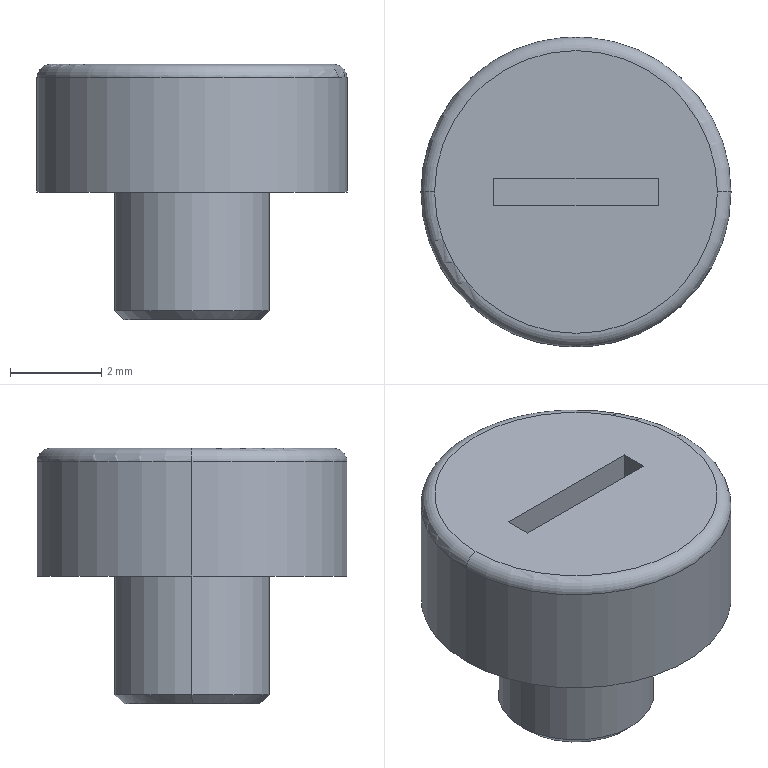Part | STEP file | 4V430C_15_Valve_Button | 1 solid | 16 faces | box 6.8 x 6.8 x 5.6 mm | volume 124.339 mm3 | plane 8 | cylinder 4 | cone 2 | torus 2 | commonest cylinder face diameters 3.4 x2 6.8 x2
STEP:
#1=CARTESIAN_POINT('',(0.,0.,0.));
#2=DIRECTION('',(0.,0.,1.));
#3=DIRECTION('',(1.,0.,0.));
#4=AXIS2_PLACEMENT_3D('',#1,#2,#3);
#5=CARTESIAN_POINT('',(1.5,0.,-2.8));
#6=VERTEX_POINT('',#5);
#7=CARTESIAN_POINT('',(-1.5,0.,-2.8));
#8=VERTEX_POINT('',#7);
#9=CARTESIAN_POINT('',(0.,0.,-2.8));
#10=DIRECTION('',(0.,0.,1.));
#11=DIRECTION('',(1.,0.,0.));
#12=AXIS2_PLACEMENT_3D('',#9,#10,#11);
#13=CIRCLE('',#12,1.5);
#14=CARTESIAN_POINT('',(0.,0.,-2.8));
#15=DIRECTION('',(0.,0.,1.));
#16=DIRECTION('',(1.,0.,0.));
#17=AXIS2_PLACEMENT_3D('',#14,#15,#16);
#18=CONICAL_SURFACE('',#17,1.5,0.7854);
#19=CARTESIAN_POINT('',(0.,0.));
#20=DIRECTION('',(1.,0.));
#21=VECTOR('',#20,1.);
#22=LINE('',#19,#21);
#23=(GEOMETRIC_REPRESENTATION_CONTEXT(2)PARAMETRIC_REPRESENTATION_CONTEXT()REPRESENTATION_CONTEXT('',''));
#24=DEFINITIONAL_REPRESENTATION('',(#22),#23);
#25=PCURVE('',#18,#24);
#26=CARTESIAN_POINT('',(0.,1.5,-2.8));
#27=DIRECTION('',(0.,0.,1.));
#28=DIRECTION('',(1.,0.,0.));
#29=AXIS2_PLACEMENT_3D('',#26,#27,#28);
#30=PLANE('',#29);
#31=CARTESIAN_POINT('',(0.,-1.5));
#32=DIRECTION('',(1.,0.));
#33=AXIS2_PLACEMENT_2D('',#31,#32);
#34=CIRCLE('',#33,1.5);
#35=(GEOMETRIC_REPRESENTATION_CONTEXT(2)PARAMETRIC_REPRESENTATION_CONTEXT()REPRESENTATION_CONTEXT('',''));
#36=DEFINITIONAL_REPRESENTATION('',(#34),#35);
#37=PCURVE('',#30,#36);
#38=SURFACE_CURVE('',#13,(#25,#37),.PCURVE_S1.);
#39=EDGE_CURVE('',#6,#8,#38,.T.);
#40=ORIENTED_EDGE('',*,*,#39,.T.);
#41=CARTESIAN_POINT('',(-1.7,0.,-2.6));
#42=VERTEX_POINT('',#41);
#43=CARTESIAN_POINT('',(-1.5,0.,-2.8));
#44=DIRECTION('',(-0.7071,0.,0.7071));
#45=VECTOR('',#44,1.);
#46=LINE('',#43,#45);
#47=CARTESIAN_POINT('',(3.142,0.));
#48=DIRECTION('',(0.,1.));
#49=VECTOR('',#48,1.);
#50=LINE('',#47,#49);
#51=(GEOMETRIC_REPRESENTATION_CONTEXT(2)PARAMETRIC_REPRESENTATION_CONTEXT()REPRESENTATION_CONTEXT('',''));
#52=DEFINITIONAL_REPRESENTATION('',(#50),#51);
#53=PCURVE('',#18,#52);
#54=CARTESIAN_POINT('',(0.,0.,-2.8));
#55=DIRECTION('',(0.,0.,1.));
#56=DIRECTION('',(1.,0.,0.));
#57=AXIS2_PLACEMENT_3D('',#54,#55,#56);
#58=CONICAL_SURFACE('',#57,1.5,0.7854);
#59=CARTESIAN_POINT('',(3.142,0.));
#60=DIRECTION('',(0.,1.));
#61=VECTOR('',#60,1.);
#62=LINE('',#59,#61);
#63=(GEOMETRIC_REPRESENTATION_CONTEXT(2)PARAMETRIC_REPRESENTATION_CONTEXT()REPRESENTATION_CONTEXT('',''));
#64=DEFINITIONAL_REPRESENTATION('',(#62),#63);
#65=PCURVE('',#58,#64);
#66=SURFACE_CURVE('',#46,(#53,#65),.PCURVE_S1.);
#67=EDGE_CURVE('',#8,#42,#66,.T.);
#68=ORIENTED_EDGE('',*,*,#67,.T.);
#69=CARTESIAN_POINT('',(1.7,0.,-2.6));
#70=VERTEX_POINT('',#69);
#71=CARTESIAN_POINT('',(0.,0.,-2.6));
#72=DIRECTION('',(0.,0.,1.));
#73=DIRECTION('',(1.,0.,0.));
#74=AXIS2_PLACEMENT_3D('',#71,#72,#73);
#75=CIRCLE('',#74,1.7);
#76=CARTESIAN_POINT('',(0.,0.2));
#77=DIRECTION('',(1.,0.));
#78=VECTOR('',#77,1.);
#79=LINE('',#76,#78);
#80=(GEOMETRIC_REPRESENTATION_CONTEXT(2)PARAMETRIC_REPRESENTATION_CONTEXT()REPRESENTATION_CONTEXT('',''));
#81=DEFINITIONAL_REPRESENTATION('',(#79),#80);
#82=PCURVE('',#18,#81);
#83=CARTESIAN_POINT('',(0.,0.,-2.8));
#84=DIRECTION('',(0.,0.,1.));
#85=DIRECTION('',(1.,0.,0.));
#86=AXIS2_PLACEMENT_3D('',#83,#84,#85);
#87=CYLINDRICAL_SURFACE('',#86,1.7);
#88=CARTESIAN_POINT('',(0.,0.2));
#89=DIRECTION('',(1.,0.));
#90=VECTOR('',#89,1.);
#91=LINE('',#88,#90);
#92=(GEOMETRIC_REPRESENTATION_CONTEXT(2)PARAMETRIC_REPRESENTATION_CONTEXT()REPRESENTATION_CONTEXT('',''));
#93=DEFINITIONAL_REPRESENTATION('',(#91),#92);
#94=PCURVE('',#87,#93);
#95=SURFACE_CURVE('',#75,(#82,#94),.PCURVE_S1.);
#96=EDGE_CURVE('',#70,#42,#95,.T.);
#97=ORIENTED_EDGE('',*,*,#96,.F.);
#98=CARTESIAN_POINT('',(1.5,0.,-2.8));
#99=DIRECTION('',(0.7071,0.,0.7071));
#100=VECTOR('',#99,1.);
#101=LINE('',#98,#100);
#102=CARTESIAN_POINT('',(0.,0.));
#103=DIRECTION('',(0.,1.));
#104=VECTOR('',#103,1.);
#105=LINE('',#102,#104);
#106=(GEOMETRIC_REPRESENTATION_CONTEXT(2)PARAMETRIC_REPRESENTATION_CONTEXT()REPRESENTATION_CONTEXT('',''));
#107=DEFINITIONAL_REPRESENTATION('',(#105),#106);
#108=PCURVE('',#18,#107);
#109=CARTESIAN_POINT('',(6.283,0.));
#110=DIRECTION('',(0.,1.));
#111=VECTOR('',#110,1.);
#112=LINE('',#109,#111);
#113=(GEOMETRIC_REPRESENTATION_CONTEXT(2)PARAMETRIC_REPRESENTATION_CONTEXT()REPRESENTATION_CONTEXT('',''));
#114=DEFINITIONAL_REPRESENTATION('',(#112),#113);
#115=PCURVE('',#58,#114);
#116=SURFACE_CURVE('',#101,(#108,#115),.PCURVE_S1.);
#117=EDGE_CURVE('',#6,#70,#116,.T.);
#118=ORIENTED_EDGE('',*,*,#117,.F.);
#119=EDGE_LOOP('',(#40,#68,#97,#118));
#120=FACE_BOUND('',#119,.T.);
#121=ADVANCED_FACE('',(#120),#18,.T.);
#122=ORIENTED_EDGE('',*,*,#96,.T.);
#123=CARTESIAN_POINT('',(-1.7,0.,0.));
#124=VERTEX_POINT('',#123);
#125=CARTESIAN_POINT('',(-1.7,0.,-2.8));
#126=DIRECTION('',(0.,0.,1.));
#127=VECTOR('',#126,1.);
#128=LINE('',#125,#127);
#129=CARTESIAN_POINT('',(3.142,0.));
#130=DIRECTION('',(0.,1.));
#131=VECTOR('',#130,1.);
#132=LINE('',#129,#131);
#133=(GEOMETRIC_REPRESENTATION_CONTEXT(2)PARAMETRIC_REPRESENTATION_CONTEXT()REPRESENTATION_CONTEXT('',''));
#134=DEFINITIONAL_REPRESENTATION('',(#132),#133);
#135=PCURVE('',#87,#134);
#136=CARTESIAN_POINT('',(0.,0.,-2.8));
#137=DIRECTION('',(0.,0.,1.));
#138=DIRECTION('',(1.,0.,0.));
#139=AXIS2_PLACEMENT_3D('',#136,#137,#138);
#140=CYLINDRICAL_SURFACE('',#139,1.7);
#141=CARTESIAN_POINT('',(3.142,0.));
#142=DIRECTION('',(0.,1.));
#143=VECTOR('',#142,1.);
#144=LINE('',#141,#143);
#145=(GEOMETRIC_REPRESENTATION_CONTEXT(2)PARAMETRIC_REPRESENTATION_CONTEXT()REPRESENTATION_CONTEXT('',''));
#146=DEFINITIONAL_REPRESENTATION('',(#144),#145);
#147=PCURVE('',#140,#146);
#148=SURFACE_CURVE('',#128,(#135,#147),.PCURVE_S1.);
#149=EDGE_CURVE('',#42,#124,#148,.T.);
#150=ORIENTED_EDGE('',*,*,#149,.T.);
#151=CARTESIAN_POINT('',(1.7,0.,0.));
#152=VERTEX_POINT('',#151);
#153=CARTESIAN_POINT('',(0.,0.,0.));
#154=DIRECTION('',(0.,0.,1.));
#155=DIRECTION('',(1.,0.,0.));
#156=AXIS2_PLACEMENT_3D('',#153,#154,#155);
#157=CIRCLE('',#156,1.7);
#158=CARTESIAN_POINT('',(0.,2.8));
#159=DIRECTION('',(1.,0.));
#160=VECTOR('',#159,1.);
#161=LINE('',#158,#160);
#162=(GEOMETRIC_REPRESENTATION_CONTEXT(2)PARAMETRIC_REPRESENTATION_CONTEXT()REPRESENTATION_CONTEXT('',''));
#163=DEFINITIONAL_REPRESENTATION('',(#161),#162);
#164=PCURVE('',#87,#163);
#165=CARTESIAN_POINT('',(0.,3.4,0.));
#166=DIRECTION('',(0.,0.,1.));
#167=DIRECTION('',(1.,0.,0.));
#168=AXIS2_PLACEMENT_3D('',#165,#166,#167);
#169=PLANE('',#168);
#170=CARTESIAN_POINT('',(0.,-3.4));
#171=DIRECTION('',(1.,0.));
#172=AXIS2_PLACEMENT_2D('',#170,#171);
#173=CIRCLE('',#172,1.7);
#174=(GEOMETRIC_REPRESENTATION_CONTEXT(2)PARAMETRIC_REPRESENTATION_CONTEXT()REPRESENTATION_CONTEXT('',''));
#175=DEFINITIONAL_REPRESENTATION('',(#173),#174);
#176=PCURVE('',#169,#175);
#177=SURFACE_CURVE('',#157,(#164,#176),.PCURVE_S1.);
#178=EDGE_CURVE('',#152,#124,#177,.T.);
#179=ORIENTED_EDGE('',*,*,#178,.F.);
#180=CARTESIAN_POINT('',(1.7,0.,-2.8));
#181=DIRECTION('',(0.,0.,1.));
#182=VECTOR('',#181,1.);
#183=LINE('',#180,#182);
#184=CARTESIAN_POINT('',(0.,0.));
#185=DIRECTION('',(0.,1.));
#186=VECTOR('',#185,1.);
#187=LINE('',#184,#186);
#188=(GEOMETRIC_REPRESENTATION_CONTEXT(2)PARAMETRIC_REPRESENTATION_CONTEXT()REPRESENTATION_CONTEXT('',''));
#189=DEFINITIONAL_REPRESENTATION('',(#187),#188);
#190=PCURVE('',#87,#189);
#191=CARTESIAN_POINT('',(6.283,0.));
#192=DIRECTION('',(0.,1.));
#193=VECTOR('',#192,1.);
#194=LINE('',#191,#193);
#195=(GEOMETRIC_REPRESENTATION_CONTEXT(2)PARAMETRIC_REPRESENTATION_CONTEXT()REPRESENTATION_CONTEXT('',''));
#196=DEFINITIONAL_REPRESENTATION('',(#194),#195);
#197=PCURVE('',#140,#196);
#198=SURFACE_CURVE('',#183,(#190,#197),.PCURVE_S1.);
#199=EDGE_CURVE('',#70,#152,#198,.T.);
#200=ORIENTED_EDGE('',*,*,#199,.F.);
#201=EDGE_LOOP('',(#122,#150,#179,#200));
#202=FACE_BOUND('',#201,.T.);
#203=ADVANCED_FACE('',(#202),#87,.T.);
#204=CARTESIAN_POINT('',(3.4,0.,0.));
#205=VERTEX_POINT('',#204);
#206=CARTESIAN_POINT('',(-3.4,0.,0.));
#207=VERTEX_POINT('',#206);
#208=CARTESIAN_POINT('',(0.,0.,0.));
#209=DIRECTION('',(0.,0.,1.));
#210=DIRECTION('',(1.,0.,0.));
#211=AXIS2_PLACEMENT_3D('',#208,#209,#210);
#212=CIRCLE('',#211,3.4);
#213=CARTESIAN_POINT('',(0.,0.,-2.8));
#214=DIRECTION('',(0.,0.,1.));
#215=DIRECTION('',(1.,0.,0.));
#216=AXIS2_PLACEMENT_3D('',#213,#214,#215);
#217=CYLINDRICAL_SURFACE('',#216,3.4);
#218=CARTESIAN_POINT('',(0.,2.8));
#219=DIRECTION('',(1.,0.));
#220=VECTOR('',#219,1.);
#221=LINE('',#218,#220);
#222=(GEOMETRIC_REPRESENTATION_CONTEXT(2)PARAMETRIC_REPRESENTATION_CONTEXT()REPRESENTATION_CONTEXT('',''));
#223=DEFINITIONAL_REPRESENTATION('',(#221),#222);
#224=PCURVE('',#217,#223);
#225=CARTESIAN_POINT('',(0.,-3.4));
#226=DIRECTION('',(1.,0.));
#227=AXIS2_PLACEMENT_2D('',#225,#226);
#228=CIRCLE('',#227,3.4);
#229=(GEOMETRIC_REPRESENTATION_CONTEXT(2)PARAMETRIC_REPRESENTATION_CONTEXT()REPRESENTATION_CONTEXT('',''));
#230=DEFINITIONAL_REPRESENTATION('',(#228),#229);
#231=PCURVE('',#169,#230);
#232=SURFACE_CURVE('',#212,(#224,#231),.PCURVE_S1.);
#233=EDGE_CURVE('',#205,#207,#232,.T.);
#234=ORIENTED_EDGE('',*,*,#233,.T.);
#235=CARTESIAN_POINT('',(-3.4,0.,2.5));
#236=VERTEX_POINT('',#235);
#237=CARTESIAN_POINT('',(-3.4,0.,-2.8));
#238=DIRECTION('',(0.,0.,1.));
#239=VECTOR('',#238,1.);
#240=LINE('',#237,#239);
#241=CARTESIAN_POINT('',(3.142,0.));
#242=DIRECTION('',(0.,1.));
#243=VECTOR('',#242,1.);
#244=LINE('',#241,#243);
#245=(GEOMETRIC_REPRESENTATION_CONTEXT(2)PARAMETRIC_REPRESENTATION_CONTEXT()REPRESENTATION_CONTEXT('',''));
#246=DEFINITIONAL_REPRESENTATION('',(#244),#245);
#247=PCURVE('',#217,#246);
#248=CARTESIAN_POINT('',(0.,0.,-2.8));
#249=DIRECTION('',(0.,0.,1.));
#250=DIRECTION('',(1.,0.,0.));
#251=AXIS2_PLACEMENT_3D('',#248,#249,#250);
#252=CYLINDRICAL_SURFACE('',#251,3.4);
#253=CARTESIAN_POINT('',(3.142,0.));
#254=DIRECTION('',(0.,1.));
#255=VECTOR('',#254,1.);
#256=LINE('',#253,#255);
#257=(GEOMETRIC_REPRESENTATION_CONTEXT(2)PARAMETRIC_REPRESENTATION_CONTEXT()REPRESENTATION_CONTEXT('',''));
#258=DEFINITIONAL_REPRESENTATION('',(#256),#257);
#259=PCURVE('',#252,#258);
#260=SURFACE_CURVE('',#240,(#247,#259),.PCURVE_S1.);
#261=EDGE_CURVE('',#207,#236,#260,.T.);
#262=ORIENTED_EDGE('',*,*,#261,.T.);
#263=CARTESIAN_POINT('',(3.4,0.,2.5));
#264=VERTEX_POINT('',#263);
#265=CARTESIAN_POINT('',(0.,0.,2.5));
#266=DIRECTION('',(0.,0.,1.));
#267=DIRECTION('',(1.,0.,0.));
#268=AXIS2_PLACEMENT_3D('',#265,#266,#267);
#269=CIRCLE('',#268,3.4);
#270=CARTESIAN_POINT('',(0.,5.3));
#271=DIRECTION('',(1.,0.));
#272=VECTOR('',#271,1.);
#273=LINE('',#270,#272);
#274=(GEOMETRIC_REPRESENTATION_CONTEXT(2)PARAMETRIC_REPRESENTATION_CONTEXT()REPRESENTATION_CONTEXT('',''));
#275=DEFINITIONAL_REPRESENTATION('',(#273),#274);
#276=PCURVE('',#217,#275);
#277=CARTESIAN_POINT('',(0.,0.,2.5));
#278=DIRECTION('',(0.,0.,1.));
#279=DIRECTION('',(1.,0.,0.));
#280=AXIS2_PLACEMENT_3D('',#277,#278,#279);
#281=TOROIDAL_SURFACE('',#280,3.1,0.3);
#282=CARTESIAN_POINT('',(0.,0.));
#283=DIRECTION('',(1.,0.));
#284=VECTOR('',#283,1.);
#285=LINE('',#282,#284);
#286=(GEOMETRIC_REPRESENTATION_CONTEXT(2)PARAMETRIC_REPRESENTATION_CONTEXT()REPRESENTATION_CONTEXT('',''));
#287=DEFINITIONAL_REPRESENTATION('',(#285),#286);
#288=PCURVE('',#281,#287);
#289=SURFACE_CURVE('',#269,(#276,#288),.PCURVE_S1.);
#290=EDGE_CURVE('',#264,#236,#289,.T.);
#291=ORIENTED_EDGE('',*,*,#290,.F.);
#292=CARTESIAN_POINT('',(3.4,0.,-2.8));
#293=DIRECTION('',(0.,0.,1.));
#294=VECTOR('',#293,1.);
#295=LINE('',#292,#294);
#296=CARTESIAN_POINT('',(0.,0.));
#297=DIRECTION('',(0.,1.));
#298=VECTOR('',#297,1.);
#299=LINE('',#296,#298);
#300=(GEOMETRIC_REPRESENTATION_CONTEXT(2)PARAMETRIC_REPRESENTATION_CONTEXT()REPRESENTATION_CONTEXT('',''));
#301=DEFINITIONAL_REPRESENTATION('',(#299),#300);
#302=PCURVE('',#217,#301);
#303=CARTESIAN_POINT('',(6.283,0.));
#304=DIRECTION('',(0.,1.));
#305=VECTOR('',#304,1.);
#306=LINE('',#303,#305);
#307=(GEOMETRIC_REPRESENTATION_CONTEXT(2)PARAMETRIC_REPRESENTATION_CONTEXT()REPRESENTATION_CONTEXT('',''));
#308=DEFINITIONAL_REPRESENTATION('',(#306),#307);
#309=PCURVE('',#252,#308);
#310=SURFACE_CURVE('',#295,(#302,#309),.PCURVE_S1.);
#311=EDGE_CURVE('',#205,#264,#310,.T.);
#312=ORIENTED_EDGE('',*,*,#311,.F.);
#313=EDGE_LOOP('',(#234,#262,#291,#312));
#314=FACE_BOUND('',#313,.T.);
#315=ADVANCED_FACE('',(#314),#217,.T.);
#316=ORIENTED_EDGE('',*,*,#290,.T.);
#317=CARTESIAN_POINT('',(-3.1,0.,2.8));
#318=VERTEX_POINT('',#317);
#319=CARTESIAN_POINT('',(-3.1,0.,2.5));
#320=DIRECTION('',(0.,1.,0.));
#321=DIRECTION('',(-1.,0.,0.));
#322=AXIS2_PLACEMENT_3D('',#319,#320,#321);
#323=CIRCLE('',#322,0.3);
#324=CARTESIAN_POINT('',(3.142,0.));
#325=DIRECTION('',(0.,1.));
#326=VECTOR('',#325,1.);
#327=LINE('',#324,#326);
#328=(GEOMETRIC_REPRESENTATION_CONTEXT(2)PARAMETRIC_REPRESENTATION_CONTEXT()REPRESENTATION_CONTEXT('',''));
#329=DEFINITIONAL_REPRESENTATION('',(#327),#328);
#330=PCURVE('',#281,#329);
#331=CARTESIAN_POINT('',(0.,0.,2.5));
#332=DIRECTION('',(0.,0.,1.));
#333=DIRECTION('',(1.,0.,0.));
#334=AXIS2_PLACEMENT_3D('',#331,#332,#333);
#335=TOROIDAL_SURFACE('',#334,3.1,0.3);
#336=CARTESIAN_POINT('',(3.142,0.));
#337=DIRECTION('',(0.,1.));
#338=VECTOR('',#337,1.);
#339=LINE('',#336,#338);
#340=(GEOMETRIC_REPRESENTATION_CONTEXT(2)PARAMETRIC_REPRESENTATION_CONTEXT()REPRESENTATION_CONTEXT('',''));
#341=DEFINITIONAL_REPRESENTATION('',(#339),#340);
#342=PCURVE('',#335,#341);
#343=SURFACE_CURVE('',#323,(#330,#342),.PCURVE_S1.);
#344=EDGE_CURVE('',#236,#318,#343,.T.);
#345=ORIENTED_EDGE('',*,*,#344,.T.);
#346=CARTESIAN_POINT('',(3.1,0.,2.8));
#347=VERTEX_POINT('',#346);
#348=CARTESIAN_POINT('',(0.,0.,2.8));
#349=DIRECTION('',(0.,0.,1.));
#350=DIRECTION('',(1.,0.,0.));
#351=AXIS2_PLACEMENT_3D('',#348,#349,#350);
#352=CIRCLE('',#351,3.1);
#353=CARTESIAN_POINT('',(0.,1.571));
#354=DIRECTION('',(1.,0.));
#355=VECTOR('',#354,1.);
#356=LINE('',#353,#355);
#357=(GEOMETRIC_REPRESENTATION_CONTEXT(2)PARAMETRIC_REPRESENTATION_CONTEXT()REPRESENTATION_CONTEXT('',''));
#358=DEFINITIONAL_REPRESENTATION('',(#356),#357);
#359=PCURVE('',#281,#358);
#360=CARTESIAN_POINT('',(0.,0.,2.8));
#361=DIRECTION('',(0.,0.,-1.));
#362=DIRECTION('',(-1.,0.,0.));
#363=AXIS2_PLACEMENT_3D('',#360,#361,#362);
#364=PLANE('',#363);
#365=CARTESIAN_POINT('',(-3.1,0.));
#366=CARTESIAN_POINT('',(-3.1,5.369));
#367=CARTESIAN_POINT('',(1.55,2.685));
#368=CARTESIAN_POINT('',(6.2,0.));
#369=CARTESIAN_POINT('',(1.55,-2.685));
#370=CARTESIAN_POINT('',(-3.1,-5.369));
#371=CARTESIAN_POINT('',(-3.1,0.));
#372=(BOUNDED_CURVE()B_SPLINE_CURVE(2,(#365,#366,#367,#368,#369,#370,#371),.UNSPECIFIED.,.T.,.F.)B_SPLINE_CURVE_WITH_KNOTS((1,2,2,2,2,1),(-2.094,0.,2.094,4.189,6.283,8.378),.UNSPECIFIED.)CURVE()GEOMETRIC_REPRESENTATION_ITEM()RATIONAL_B_SPLINE_CURVE((1.,0.5,1.,0.5,1.,0.5,1.))REPRESENTATION_ITEM(''));
#373=(GEOMETRIC_REPRESENTATION_CONTEXT(2)PARAMETRIC_REPRESENTATION_CONTEXT()REPRESENTATION_CONTEXT('',''));
#374=DEFINITIONAL_REPRESENTATION('',(#372),#373);
#375=PCURVE('',#364,#374);
#376=SURFACE_CURVE('',#352,(#359,#375),.PCURVE_S1.);
#377=EDGE_CURVE('',#347,#318,#376,.T.);
#378=ORIENTED_EDGE('',*,*,#377,.F.);
#379=CARTESIAN_POINT('',(3.1,0.,2.5));
#380=DIRECTION('',(0.,-1.,0.));
#381=DIRECTION('',(0.,0.,-1.));
#382=AXIS2_PLACEMENT_3D('',#379,#380,#381);
#383=CIRCLE('',#382,0.3);
#384=CARTESIAN_POINT('',(0.,-1.571));
#385=DIRECTION('',(0.,1.));
#386=VECTOR('',#385,1.);
#387=LINE('',#384,#386);
#388=(GEOMETRIC_REPRESENTATION_CONTEXT(2)PARAMETRIC_REPRESENTATION_CONTEXT()REPRESENTATION_CONTEXT('',''));
#389=DEFINITIONAL_REPRESENTATION('',(#387),#388);
#390=PCURVE('',#281,#389);
#391=CARTESIAN_POINT('',(6.283,-1.571));
#392=DIRECTION('',(0.,1.));
#393=VECTOR('',#392,1.);
#394=LINE('',#391,#393);
#395=(GEOMETRIC_REPRESENTATION_CONTEXT(2)PARAMETRIC_REPRESENTATION_CONTEXT()REPRESENTATION_CONTEXT('',''));
#396=DEFINITIONAL_REPRESENTATION('',(#394),#395);
#397=PCURVE('',#335,#396);
#398=SURFACE_CURVE('',#383,(#390,#397),.PCURVE_S1.);
#399=EDGE_CURVE('',#264,#347,#398,.T.);
#400=ORIENTED_EDGE('',*,*,#399,.F.);
#401=EDGE_LOOP('',(#316,#345,#378,#400));
#402=FACE_BOUND('',#401,.T.);
#403=ADVANCED_FACE('',(#402),#281,.T.);
#404=ORIENTED_EDGE('',*,*,#377,.T.);
#405=CARTESIAN_POINT('',(0.,0.,2.8));
#406=DIRECTION('',(0.,0.,1.));
#407=DIRECTION('',(1.,0.,0.));
#408=AXIS2_PLACEMENT_3D('',#405,#406,#407);
#409=CIRCLE('',#408,3.1);
#410=CARTESIAN_POINT('',(-3.1,0.));
#411=CARTESIAN_POINT('',(-3.1,5.369));
#412=CARTESIAN_POINT('',(1.55,2.685));
#413=CARTESIAN_POINT('',(6.2,0.));
#414=CARTESIAN_POINT('',(1.55,-2.685));
#415=CARTESIAN_POINT('',(-3.1,-5.369));
#416=CARTESIAN_POINT('',(-3.1,0.));
#417=(BOUNDED_CURVE()B_SPLINE_CURVE(2,(#410,#411,#412,#413,#414,#415,#416),.UNSPECIFIED.,.T.,.F.)B_SPLINE_CURVE_WITH_KNOTS((1,2,2,2,2,1),(-2.094,0.,2.094,4.189,6.283,8.378),.UNSPECIFIED.)CURVE()GEOMETRIC_REPRESENTATION_ITEM()RATIONAL_B_SPLINE_CURVE((1.,0.5,1.,0.5,1.,0.5,1.))REPRESENTATION_ITEM(''));
#418=(GEOMETRIC_REPRESENTATION_CONTEXT(2)PARAMETRIC_REPRESENTATION_CONTEXT()REPRESENTATION_CONTEXT('',''));
#419=DEFINITIONAL_REPRESENTATION('',(#417),#418);
#420=PCURVE('',#364,#419);
#421=CARTESIAN_POINT('',(0.,1.571));
#422=DIRECTION('',(1.,0.));
#423=VECTOR('',#422,1.);
#424=LINE('',#421,#423);
#425=(GEOMETRIC_REPRESENTATION_CONTEXT(2)PARAMETRIC_REPRESENTATION_CONTEXT()REPRESENTATION_CONTEXT('',''));
#426=DEFINITIONAL_REPRESENTATION('',(#424),#425);
#427=PCURVE('',#335,#426);
#428=SURFACE_CURVE('',#409,(#420,#427),.PCURVE_S1.);
#429=EDGE_CURVE('',#318,#347,#428,.T.);
#430=ORIENTED_EDGE('',*,*,#429,.T.);
#431=EDGE_LOOP('',(#404,#430));
#432=FACE_BOUND('',#431,.T.);
#433=CARTESIAN_POINT('',(-1.8,0.3,2.8));
#434=VERTEX_POINT('',#433);
#435=CARTESIAN_POINT('',(-1.8,-0.3,2.8));
#436=VERTEX_POINT('',#435);
#437=CARTESIAN_POINT('',(-1.8,0.3,2.8));
#438=DIRECTION('',(0.,-1.,0.));
#439=VECTOR('',#438,1.);
#440=LINE('',#437,#439);
#441=CARTESIAN_POINT('',(1.8,0.3));
#442=DIRECTION('',(0.,-1.));
#443=VECTOR('',#442,1.);
#444=LINE('',#441,#443);
#445=(GEOMETRIC_REPRESENTATION_CONTEXT(2)PARAMETRIC_REPRESENTATION_CONTEXT()REPRESENTATION_CONTEXT('',''));
#446=DEFINITIONAL_REPRESENTATION('',(#444),#445);
#447=PCURVE('',#364,#446);
#448=CARTESIAN_POINT('',(-1.8,-0.3,2.8));
#449=DIRECTION('',(1.,0.,0.));
#450=DIRECTION('',(0.,0.,-1.));
#451=AXIS2_PLACEMENT_3D('',#448,#449,#450);
#452=PLANE('',#451);
#453=CARTESIAN_POINT('',(0.,0.6));
#454=DIRECTION('',(0.,-1.));
#455=VECTOR('',#454,1.);
#456=LINE('',#453,#455);
#457=(GEOMETRIC_REPRESENTATION_CONTEXT(2)PARAMETRIC_REPRESENTATION_CONTEXT()REPRESENTATION_CONTEXT('',''));
#458=DEFINITIONAL_REPRESENTATION('',(#456),#457);
#459=PCURVE('',#452,#458);
#460=SURFACE_CURVE('',#440,(#447,#459),.PCURVE_S1.);
#461=EDGE_CURVE('',#434,#436,#460,.T.);
#462=ORIENTED_EDGE('',*,*,#461,.F.);
#463=CARTESIAN_POINT('',(1.8,0.3,2.8));
#464=VERTEX_POINT('',#463);
#465=CARTESIAN_POINT('',(-1.8,0.3,2.8));
#466=DIRECTION('',(1.,0.,0.));
#467=VECTOR('',#466,1.);
#468=LINE('',#465,#467);
#469=CARTESIAN_POINT('',(1.8,0.3));
#470=DIRECTION('',(-1.,0.));
#471=VECTOR('',#470,1.);
#472=LINE('',#469,#471);
#473=(GEOMETRIC_REPRESENTATION_CONTEXT(2)PARAMETRIC_REPRESENTATION_CONTEXT()REPRESENTATION_CONTEXT('',''));
#474=DEFINITIONAL_REPRESENTATION('',(#472),#473);
#475=PCURVE('',#364,#474);
#476=CARTESIAN_POINT('',(-1.8,0.3,1.8));
#477=DIRECTION('',(0.,1.,0.));
#478=DIRECTION('',(0.,0.,1.));
#479=AXIS2_PLACEMENT_3D('',#476,#477,#478);
#480=PLANE('',#479);
#481=CARTESIAN_POINT('',(1.,0.));
#482=DIRECTION('',(0.,1.));
#483=VECTOR('',#482,1.);
#484=LINE('',#481,#483);
#485=(GEOMETRIC_REPRESENTATION_CONTEXT(2)PARAMETRIC_REPRESENTATION_CONTEXT()REPRESENTATION_CONTEXT('',''));
#486=DEFINITIONAL_REPRESENTATION('',(#484),#485);
#487=PCURVE('',#480,#486);
#488=SURFACE_CURVE('',#468,(#475,#487),.PCURVE_S1.);
#489=EDGE_CURVE('',#434,#464,#488,.T.);
#490=ORIENTED_EDGE('',*,*,#489,.T.);
#491=CARTESIAN_POINT('',(1.8,-0.3,2.8));
#492=VERTEX_POINT('',#491);
#493=CARTESIAN_POINT('',(1.8,0.3,2.8));
#494=DIRECTION('',(0.,-1.,0.));
#495=VECTOR('',#494,1.);
#496=LINE('',#493,#495);
#497=CARTESIAN_POINT('',(-1.8,0.3));
#498=DIRECTION('',(0.,-1.));
#499=VECTOR('',#498,1.);
#500=LINE('',#497,#499);
#501=(GEOMETRIC_REPRESENTATION_CONTEXT(2)PARAMETRIC_REPRESENTATION_CONTEXT()REPRESENTATION_CONTEXT('',''));
#502=DEFINITIONAL_REPRESENTATION('',(#500),#501);
#503=PCURVE('',#364,#502);
#504=CARTESIAN_POINT('',(1.8,-0.3,2.8));
#505=DIRECTION('',(1.,0.,0.));
#506=DIRECTION('',(0.,0.,-1.));
#507=AXIS2_PLACEMENT_3D('',#504,#505,#506);
#508=PLANE('',#507);
#509=CARTESIAN_POINT('',(0.,0.6));
#510=DIRECTION('',(0.,-1.));
#511=VECTOR('',#510,1.);
#512=LINE('',#509,#511);
#513=(GEOMETRIC_REPRESENTATION_CONTEXT(2)PARAMETRIC_REPRESENTATION_CONTEXT()REPRESENTATION_CONTEXT('',''));
#514=DEFINITIONAL_REPRESENTATION('',(#512),#513);
#515=PCURVE('',#508,#514);
#516=SURFACE_CURVE('',#496,(#503,#515),.PCURVE_S1.);
#517=EDGE_CURVE('',#464,#492,#516,.T.);
#518=ORIENTED_EDGE('',*,*,#517,.T.);
#519=CARTESIAN_POINT('',(-1.8,-0.3,2.8));
#520=DIRECTION('',(1.,0.,0.));
#521=VECTOR('',#520,1.);
#522=LINE('',#519,#521);
#523=CARTESIAN_POINT('',(1.8,-0.3));
#524=DIRECTION('',(-1.,0.));
#525=VECTOR('',#524,1.);
#526=LINE('',#523,#525);
#527=(GEOMETRIC_REPRESENTATION_CONTEXT(2)PARAMETRIC_REPRESENTATION_CONTEXT()REPRESENTATION_CONTEXT('',''));
#528=DEFINITIONAL_REPRESENTATION('',(#526),#527);
#529=PCURVE('',#364,#528);
#530=CARTESIAN_POINT('',(-1.8,-0.3,2.8));
#531=DIRECTION('',(0.,-1.,0.));
#532=DIRECTION('',(0.,0.,-1.));
#533=AXIS2_PLACEMENT_3D('',#530,#531,#532);
#534=PLANE('',#533);
#535=CARTESIAN_POINT('',(0.,0.));
#536=DIRECTION('',(0.,1.));
#537=VECTOR('',#536,1.);
#538=LINE('',#535,#537);
#539=(GEOMETRIC_REPRESENTATION_CONTEXT(2)PARAMETRIC_REPRESENTATION_CONTEXT()REPRESENTATION_CONTEXT('',''));
#540=DEFINITIONAL_REPRESENTATION('',(#538),#539);
#541=PCURVE('',#534,#540);
#542=SURFACE_CURVE('',#522,(#529,#541),.PCURVE_S1.);
#543=EDGE_CURVE('',#436,#492,#542,.T.);
#544=ORIENTED_EDGE('',*,*,#543,.F.);
#545=EDGE_LOOP('',(#462,#490,#518,#544));
#546=FACE_BOUND('',#545,.T.);
#547=ADVANCED_FACE('',(#432,#546),#364,.F.);
#548=ORIENTED_EDGE('',*,*,#344,.F.);
#549=CARTESIAN_POINT('',(0.,0.,2.5));
#550=DIRECTION('',(0.,0.,1.));
#551=DIRECTION('',(1.,0.,0.));
#552=AXIS2_PLACEMENT_3D('',#549,#550,#551);
#553=CIRCLE('',#552,3.4);
#554=CARTESIAN_POINT('',(0.,0.));
#555=DIRECTION('',(1.,0.));
#556=VECTOR('',#555,1.);
#557=LINE('',#554,#556);
#558=(GEOMETRIC_REPRESENTATION_CONTEXT(2)PARAMETRIC_REPRESENTATION_CONTEXT()REPRESENTATION_CONTEXT('',''));
#559=DEFINITIONAL_REPRESENTATION('',(#557),#558);
#560=PCURVE('',#335,#559);
#561=CARTESIAN_POINT('',(0.,5.3));
#562=DIRECTION('',(1.,0.));
#563=VECTOR('',#562,1.);
#564=LINE('',#561,#563);
#565=(GEOMETRIC_REPRESENTATION_CONTEXT(2)PARAMETRIC_REPRESENTATION_CONTEXT()REPRESENTATION_CONTEXT('',''));
#566=DEFINITIONAL_REPRESENTATION('',(#564),#565);
#567=PCURVE('',#252,#566);
#568=SURFACE_CURVE('',#553,(#560,#567),.PCURVE_S1.);
#569=EDGE_CURVE('',#236,#264,#568,.T.);
#570=ORIENTED_EDGE('',*,*,#569,.T.);
#571=ORIENTED_EDGE('',*,*,#399,.T.);
#572=ORIENTED_EDGE('',*,*,#429,.F.);
#573=EDGE_LOOP('',(#548,#570,#571,#572));
#574=FACE_BOUND('',#573,.T.);
#575=ADVANCED_FACE('',(#574),#335,.T.);
#576=ORIENTED_EDGE('',*,*,#261,.F.);
#577=CARTESIAN_POINT('',(0.,0.,0.));
#578=DIRECTION('',(0.,0.,1.));
#579=DIRECTION('',(1.,0.,0.));
#580=AXIS2_PLACEMENT_3D('',#577,#578,#579);
#581=CIRCLE('',#580,3.4);
#582=CARTESIAN_POINT('',(0.,2.8));
#583=DIRECTION('',(1.,0.));
#584=VECTOR('',#583,1.);
#585=LINE('',#582,#584);
#586=(GEOMETRIC_REPRESENTATION_CONTEXT(2)PARAMETRIC_REPRESENTATION_CONTEXT()REPRESENTATION_CONTEXT('',''));
#587=DEFINITIONAL_REPRESENTATION('',(#585),#586);
#588=PCURVE('',#252,#587);
#589=CARTESIAN_POINT('',(0.,-3.4));
#590=DIRECTION('',(1.,0.));
#591=AXIS2_PLACEMENT_2D('',#589,#590);
#592=CIRCLE('',#591,3.4);
#593=(GEOMETRIC_REPRESENTATION_CONTEXT(2)PARAMETRIC_REPRESENTATION_CONTEXT()REPRESENTATION_CONTEXT('',''));
#594=DEFINITIONAL_REPRESENTATION('',(#592),#593);
#595=PCURVE('',#169,#594);
#596=SURFACE_CURVE('',#581,(#588,#595),.PCURVE_S1.);
#597=EDGE_CURVE('',#207,#205,#596,.T.);
#598=ORIENTED_EDGE('',*,*,#597,.T.);
#599=ORIENTED_EDGE('',*,*,#311,.T.);
#600=ORIENTED_EDGE('',*,*,#569,.F.);
#601=EDGE_LOOP('',(#576,#598,#599,#600));
#602=FACE_BOUND('',#601,.T.);
#603=ADVANCED_FACE('',(#602),#252,.T.);
#604=ORIENTED_EDGE('',*,*,#233,.F.);
#605=ORIENTED_EDGE('',*,*,#597,.F.);
#606=EDGE_LOOP('',(#604,#605));
#607=FACE_BOUND('',#606,.T.);
#608=ORIENTED_EDGE('',*,*,#178,.T.);
#609=CARTESIAN_POINT('',(0.,0.,0.));
#610=DIRECTION('',(0.,0.,1.));
#611=DIRECTION('',(1.,0.,0.));
#612=AXIS2_PLACEMENT_3D('',#609,#610,#611);
#613=CIRCLE('',#612,1.7);
#614=CARTESIAN_POINT('',(0.,-3.4));
#615=DIRECTION('',(1.,0.));
#616=AXIS2_PLACEMENT_2D('',#614,#615);
#617=CIRCLE('',#616,1.7);
#618=(GEOMETRIC_REPRESENTATION_CONTEXT(2)PARAMETRIC_REPRESENTATION_CONTEXT()REPRESENTATION_CONTEXT('',''));
#619=DEFINITIONAL_REPRESENTATION('',(#617),#618);
#620=PCURVE('',#169,#619);
#621=CARTESIAN_POINT('',(0.,2.8));
#622=DIRECTION('',(1.,0.));
#623=VECTOR('',#622,1.);
#624=LINE('',#621,#623);
#625=(GEOMETRIC_REPRESENTATION_CONTEXT(2)PARAMETRIC_REPRESENTATION_CONTEXT()REPRESENTATION_CONTEXT('',''));
#626=DEFINITIONAL_REPRESENTATION('',(#624),#625);
#627=PCURVE('',#140,#626);
#628=SURFACE_CURVE('',#613,(#620,#627),.PCURVE_S1.);
#629=EDGE_CURVE('',#124,#152,#628,.T.);
#630=ORIENTED_EDGE('',*,*,#629,.T.);
#631=EDGE_LOOP('',(#608,#630));
#632=FACE_BOUND('',#631,.T.);
#633=ADVANCED_FACE('',(#607,#632),#169,.F.);
#634=ORIENTED_EDGE('',*,*,#149,.F.);
#635=CARTESIAN_POINT('',(0.,0.,-2.6));
#636=DIRECTION('',(0.,0.,1.));
#637=DIRECTION('',(1.,0.,0.));
#638=AXIS2_PLACEMENT_3D('',#635,#636,#637);
#639=CIRCLE('',#638,1.7);
#640=CARTESIAN_POINT('',(0.,0.2));
#641=DIRECTION('',(1.,0.));
#642=VECTOR('',#641,1.);
#643=LINE('',#640,#642);
#644=(GEOMETRIC_REPRESENTATION_CONTEXT(2)PARAMETRIC_REPRESENTATION_CONTEXT()REPRESENTATION_CONTEXT('',''));
#645=DEFINITIONAL_REPRESENTATION('',(#643),#644);
#646=PCURVE('',#140,#645);
#647=CARTESIAN_POINT('',(0.,0.2));
#648=DIRECTION('',(1.,0.));
#649=VECTOR('',#648,1.);
#650=LINE('',#647,#649);
#651=(GEOMETRIC_REPRESENTATION_CONTEXT(2)PARAMETRIC_REPRESENTATION_CONTEXT()REPRESENTATION_CONTEXT('',''));
#652=DEFINITIONAL_REPRESENTATION('',(#650),#651);
#653=PCURVE('',#58,#652);
#654=SURFACE_CURVE('',#639,(#646,#653),.PCURVE_S1.);
#655=EDGE_CURVE('',#42,#70,#654,.T.);
#656=ORIENTED_EDGE('',*,*,#655,.T.);
#657=ORIENTED_EDGE('',*,*,#199,.T.);
#658=ORIENTED_EDGE('',*,*,#629,.F.);
#659=EDGE_LOOP('',(#634,#656,#657,#658));
#660=FACE_BOUND('',#659,.T.);
#661=ADVANCED_FACE('',(#660),#140,.T.);
#662=ORIENTED_EDGE('',*,*,#67,.F.);
#663=CARTESIAN_POINT('',(0.,0.,-2.8));
#664=DIRECTION('',(0.,0.,1.));
#665=DIRECTION('',(1.,0.,0.));
#666=AXIS2_PLACEMENT_3D('',#663,#664,#665);
#667=CIRCLE('',#666,1.5);
#668=CARTESIAN_POINT('',(0.,0.));
#669=DIRECTION('',(1.,0.));
#670=VECTOR('',#669,1.);
#671=LINE('',#668,#670);
#672=(GEOMETRIC_REPRESENTATION_CONTEXT(2)PARAMETRIC_REPRESENTATION_CONTEXT()REPRESENTATION_CONTEXT('',''));
#673=DEFINITIONAL_REPRESENTATION('',(#671),#672);
#674=PCURVE('',#58,#673);
#675=CARTESIAN_POINT('',(0.,-1.5));
#676=DIRECTION('',(1.,0.));
#677=AXIS2_PLACEMENT_2D('',#675,#676);
#678=CIRCLE('',#677,1.5);
#679=(GEOMETRIC_REPRESENTATION_CONTEXT(2)PARAMETRIC_REPRESENTATION_CONTEXT()REPRESENTATION_CONTEXT('',''));
#680=DEFINITIONAL_REPRESENTATION('',(#678),#679);
#681=PCURVE('',#30,#680);
#682=SURFACE_CURVE('',#667,(#674,#681),.PCURVE_S1.);
#683=EDGE_CURVE('',#8,#6,#682,.T.);
#684=ORIENTED_EDGE('',*,*,#683,.T.);
#685=ORIENTED_EDGE('',*,*,#117,.T.);
#686=ORIENTED_EDGE('',*,*,#655,.F.);
#687=EDGE_LOOP('',(#662,#684,#685,#686));
#688=FACE_BOUND('',#687,.T.);
#689=ADVANCED_FACE('',(#688),#58,.T.);
#690=ORIENTED_EDGE('',*,*,#39,.F.);
#691=ORIENTED_EDGE('',*,*,#683,.F.);
#692=EDGE_LOOP('',(#690,#691));
#693=FACE_BOUND('',#692,.T.);
#694=ADVANCED_FACE('',(#693),#30,.F.);
#695=ORIENTED_EDGE('',*,*,#489,.F.);
#696=CARTESIAN_POINT('',(-1.8,0.3,1.8));
#697=VERTEX_POINT('',#696);
#698=CARTESIAN_POINT('',(-1.8,0.3,1.8));
#699=DIRECTION('',(0.,0.,1.));
#700=VECTOR('',#699,1.);
#701=LINE('',#698,#700);
#702=CARTESIAN_POINT('',(0.,0.));
#703=DIRECTION('',(1.,0.));
#704=VECTOR('',#703,1.);
#705=LINE('',#702,#704);
#706=(GEOMETRIC_REPRESENTATION_CONTEXT(2)PARAMETRIC_REPRESENTATION_CONTEXT()REPRESENTATION_CONTEXT('',''));
#707=DEFINITIONAL_REPRESENTATION('',(#705),#706);
#708=PCURVE('',#480,#707);
#709=CARTESIAN_POINT('',(1.,0.6));
#710=DIRECTION('',(-1.,0.));
#711=VECTOR('',#710,1.);
#712=LINE('',#709,#711);
#713=(GEOMETRIC_REPRESENTATION_CONTEXT(2)PARAMETRIC_REPRESENTATION_CONTEXT()REPRESENTATION_CONTEXT('',''));
#714=DEFINITIONAL_REPRESENTATION('',(#712),#713);
#715=PCURVE('',#452,#714);
#716=SURFACE_CURVE('',#701,(#708,#715),.PCURVE_S1.);
#717=EDGE_CURVE('',#697,#434,#716,.T.);
#718=ORIENTED_EDGE('',*,*,#717,.F.);
#719=CARTESIAN_POINT('',(1.8,0.3,1.8));
#720=VERTEX_POINT('',#719);
#721=CARTESIAN_POINT('',(-1.8,0.3,1.8));
#722=DIRECTION('',(1.,0.,0.));
#723=VECTOR('',#722,1.);
#724=LINE('',#721,#723);
#725=CARTESIAN_POINT('',(0.,0.));
#726=DIRECTION('',(0.,1.));
#727=VECTOR('',#726,1.);
#728=LINE('',#725,#727);
#729=(GEOMETRIC_REPRESENTATION_CONTEXT(2)PARAMETRIC_REPRESENTATION_CONTEXT()REPRESENTATION_CONTEXT('',''));
#730=DEFINITIONAL_REPRESENTATION('',(#728),#729);
#731=PCURVE('',#480,#730);
#732=CARTESIAN_POINT('',(-1.8,-0.3,1.8));
#733=DIRECTION('',(0.,0.,-1.));
#734=DIRECTION('',(-1.,0.,0.));
#735=AXIS2_PLACEMENT_3D('',#732,#733,#734);
#736=PLANE('',#735);
#737=CARTESIAN_POINT('',(0.,0.6));
#738=DIRECTION('',(-1.,0.));
#739=VECTOR('',#738,1.);
#740=LINE('',#737,#739);
#741=(GEOMETRIC_REPRESENTATION_CONTEXT(2)PARAMETRIC_REPRESENTATION_CONTEXT()REPRESENTATION_CONTEXT('',''));
#742=DEFINITIONAL_REPRESENTATION('',(#740),#741);
#743=PCURVE('',#736,#742);
#744=SURFACE_CURVE('',#724,(#731,#743),.PCURVE_S1.);
#745=EDGE_CURVE('',#697,#720,#744,.T.);
#746=ORIENTED_EDGE('',*,*,#745,.T.);
#747=CARTESIAN_POINT('',(1.8,0.3,1.8));
#748=DIRECTION('',(0.,0.,1.));
#749=VECTOR('',#748,1.);
#750=LINE('',#747,#749);
#751=CARTESIAN_POINT('',(0.,3.6));
#752=DIRECTION('',(1.,0.));
#753=VECTOR('',#752,1.);
#754=LINE('',#751,#753);
#755=(GEOMETRIC_REPRESENTATION_CONTEXT(2)PARAMETRIC_REPRESENTATION_CONTEXT()REPRESENTATION_CONTEXT('',''));
#756=DEFINITIONAL_REPRESENTATION('',(#754),#755);
#757=PCURVE('',#480,#756);
#758=CARTESIAN_POINT('',(1.,0.6));
#759=DIRECTION('',(-1.,0.));
#760=VECTOR('',#759,1.);
#761=LINE('',#758,#760);
#762=(GEOMETRIC_REPRESENTATION_CONTEXT(2)PARAMETRIC_REPRESENTATION_CONTEXT()REPRESENTATION_CONTEXT('',''));
#763=DEFINITIONAL_REPRESENTATION('',(#761),#762);
#764=PCURVE('',#508,#763);
#765=SURFACE_CURVE('',#750,(#757,#764),.PCURVE_S1.);
#766=EDGE_CURVE('',#720,#464,#765,.T.);
#767=ORIENTED_EDGE('',*,*,#766,.T.);
#768=EDGE_LOOP('',(#695,#718,#746,#767));
#769=FACE_BOUND('',#768,.T.);
#770=ADVANCED_FACE('',(#769),#480,.F.);
#771=ORIENTED_EDGE('',*,*,#745,.F.);
#772=CARTESIAN_POINT('',(-1.8,-0.3,1.8));
#773=VERTEX_POINT('',#772);
#774=CARTESIAN_POINT('',(-1.8,-0.3,1.8));
#775=DIRECTION('',(0.,1.,0.));
#776=VECTOR('',#775,1.);
#777=LINE('',#774,#776);
#778=CARTESIAN_POINT('',(0.,0.));
#779=DIRECTION('',(0.,1.));
#780=VECTOR('',#779,1.);
#781=LINE('',#778,#780);
#782=(GEOMETRIC_REPRESENTATION_CONTEXT(2)PARAMETRIC_REPRESENTATION_CONTEXT()REPRESENTATION_CONTEXT('',''));
#783=DEFINITIONAL_REPRESENTATION('',(#781),#782);
#784=PCURVE('',#736,#783);
#785=CARTESIAN_POINT('',(1.,0.));
#786=DIRECTION('',(0.,1.));
#787=VECTOR('',#786,1.);
#788=LINE('',#785,#787);
#789=(GEOMETRIC_REPRESENTATION_CONTEXT(2)PARAMETRIC_REPRESENTATION_CONTEXT()REPRESENTATION_CONTEXT('',''));
#790=DEFINITIONAL_REPRESENTATION('',(#788),#789);
#791=PCURVE('',#452,#790);
#792=SURFACE_CURVE('',#777,(#784,#791),.PCURVE_S1.);
#793=EDGE_CURVE('',#773,#697,#792,.T.);
#794=ORIENTED_EDGE('',*,*,#793,.F.);
#795=CARTESIAN_POINT('',(1.8,-0.3,1.8));
#796=VERTEX_POINT('',#795);
#797=CARTESIAN_POINT('',(-1.8,-0.3,1.8));
#798=DIRECTION('',(1.,0.,0.));
#799=VECTOR('',#798,1.);
#800=LINE('',#797,#799);
#801=CARTESIAN_POINT('',(0.,0.));
#802=DIRECTION('',(-1.,0.));
#803=VECTOR('',#802,1.);
#804=LINE('',#801,#803);
#805=(GEOMETRIC_REPRESENTATION_CONTEXT(2)PARAMETRIC_REPRESENTATION_CONTEXT()REPRESENTATION_CONTEXT('',''));
#806=DEFINITIONAL_REPRESENTATION('',(#804),#805);
#807=PCURVE('',#736,#806);
#808=CARTESIAN_POINT('',(1.,0.));
#809=DIRECTION('',(0.,1.));
#810=VECTOR('',#809,1.);
#811=LINE('',#808,#810);
#812=(GEOMETRIC_REPRESENTATION_CONTEXT(2)PARAMETRIC_REPRESENTATION_CONTEXT()REPRESENTATION_CONTEXT('',''));
#813=DEFINITIONAL_REPRESENTATION('',(#811),#812);
#814=PCURVE('',#534,#813);
#815=SURFACE_CURVE('',#800,(#807,#814),.PCURVE_S1.);
#816=EDGE_CURVE('',#773,#796,#815,.T.);
#817=ORIENTED_EDGE('',*,*,#816,.T.);
#818=CARTESIAN_POINT('',(1.8,-0.3,1.8));
#819=DIRECTION('',(0.,1.,0.));
#820=VECTOR('',#819,1.);
#821=LINE('',#818,#820);
#822=CARTESIAN_POINT('',(-3.6,0.));
#823=DIRECTION('',(0.,1.));
#824=VECTOR('',#823,1.);
#825=LINE('',#822,#824);
#826=(GEOMETRIC_REPRESENTATION_CONTEXT(2)PARAMETRIC_REPRESENTATION_CONTEXT()REPRESENTATION_CONTEXT('',''));
#827=DEFINITIONAL_REPRESENTATION('',(#825),#826);
#828=PCURVE('',#736,#827);
#829=CARTESIAN_POINT('',(1.,0.));
#830=DIRECTION('',(0.,1.));
#831=VECTOR('',#830,1.);
#832=LINE('',#829,#831);
#833=(GEOMETRIC_REPRESENTATION_CONTEXT(2)PARAMETRIC_REPRESENTATION_CONTEXT()REPRESENTATION_CONTEXT('',''));
#834=DEFINITIONAL_REPRESENTATION('',(#832),#833);
#835=PCURVE('',#508,#834);
#836=SURFACE_CURVE('',#821,(#828,#835),.PCURVE_S1.);
#837=EDGE_CURVE('',#796,#720,#836,.T.);
#838=ORIENTED_EDGE('',*,*,#837,.T.);
#839=EDGE_LOOP('',(#771,#794,#817,#838));
#840=FACE_BOUND('',#839,.T.);
#841=ADVANCED_FACE('',(#840),#736,.F.);
#842=ORIENTED_EDGE('',*,*,#816,.F.);
#843=CARTESIAN_POINT('',(-1.8,-0.3,2.8));
#844=DIRECTION('',(0.,0.,-1.));
#845=VECTOR('',#844,1.);
#846=LINE('',#843,#845);
#847=CARTESIAN_POINT('',(0.,0.));
#848=DIRECTION('',(1.,0.));
#849=VECTOR('',#848,1.);
#850=LINE('',#847,#849);
#851=(GEOMETRIC_REPRESENTATION_CONTEXT(2)PARAMETRIC_REPRESENTATION_CONTEXT()REPRESENTATION_CONTEXT('',''));
#852=DEFINITIONAL_REPRESENTATION('',(#850),#851);
#853=PCURVE('',#534,#852);
#854=CARTESIAN_POINT('',(0.,0.));
#855=DIRECTION('',(1.,0.));
#856=VECTOR('',#855,1.);
#857=LINE('',#854,#856);
#858=(GEOMETRIC_REPRESENTATION_CONTEXT(2)PARAMETRIC_REPRESENTATION_CONTEXT()REPRESENTATION_CONTEXT('',''));
#859=DEFINITIONAL_REPRESENTATION('',(#857),#858);
#860=PCURVE('',#452,#859);
#861=SURFACE_CURVE('',#846,(#853,#860),.PCURVE_S1.);
#862=EDGE_CURVE('',#436,#773,#861,.T.);
#863=ORIENTED_EDGE('',*,*,#862,.F.);
#864=ORIENTED_EDGE('',*,*,#543,.T.);
#865=CARTESIAN_POINT('',(1.8,-0.3,2.8));
#866=DIRECTION('',(0.,0.,-1.));
#867=VECTOR('',#866,1.);
#868=LINE('',#865,#867);
#869=CARTESIAN_POINT('',(0.,3.6));
#870=DIRECTION('',(1.,0.));
#871=VECTOR('',#870,1.);
#872=LINE('',#869,#871);
#873=(GEOMETRIC_REPRESENTATION_CONTEXT(2)PARAMETRIC_REPRESENTATION_CONTEXT()REPRESENTATION_CONTEXT('',''));
#874=DEFINITIONAL_REPRESENTATION('',(#872),#873);
#875=PCURVE('',#534,#874);
#876=CARTESIAN_POINT('',(0.,0.));
#877=DIRECTION('',(1.,0.));
#878=VECTOR('',#877,1.);
#879=LINE('',#876,#878);
#880=(GEOMETRIC_REPRESENTATION_CONTEXT(2)PARAMETRIC_REPRESENTATION_CONTEXT()REPRESENTATION_CONTEXT('',''));
#881=DEFINITIONAL_REPRESENTATION('',(#879),#880);
#882=PCURVE('',#508,#881);
#883=SURFACE_CURVE('',#868,(#875,#882),.PCURVE_S1.);
#884=EDGE_CURVE('',#492,#796,#883,.T.);
#885=ORIENTED_EDGE('',*,*,#884,.T.);
#886=EDGE_LOOP('',(#842,#863,#864,#885));
#887=FACE_BOUND('',#886,.T.);
#888=ADVANCED_FACE('',(#887),#534,.F.);
#889=ORIENTED_EDGE('',*,*,#461,.T.);
#890=ORIENTED_EDGE('',*,*,#862,.T.);
#891=ORIENTED_EDGE('',*,*,#793,.T.);
#892=ORIENTED_EDGE('',*,*,#717,.T.);
#893=EDGE_LOOP('',(#889,#890,#891,#892));
#894=FACE_BOUND('',#893,.T.);
#895=ADVANCED_FACE('',(#894),#452,.T.);
#896=ORIENTED_EDGE('',*,*,#517,.F.);
#897=ORIENTED_EDGE('',*,*,#766,.F.);
#898=ORIENTED_EDGE('',*,*,#837,.F.);
#899=ORIENTED_EDGE('',*,*,#884,.F.);
#900=EDGE_LOOP('',(#896,#897,#898,#899));
#901=FACE_BOUND('',#900,.T.);
#902=ADVANCED_FACE('',(#901),#508,.F.);
#903=CLOSED_SHELL('',(#121,#203,#315,#403,#547,#575,#603,#633,#661,#689,#694,#770,#841,#888,#895,#902));
#904=MANIFOLD_SOLID_BREP('',#903);
#905=(LENGTH_UNIT()NAMED_UNIT(*)SI_UNIT(.MILLI.,.METRE.));
#906=UNCERTAINTY_MEASURE_WITH_UNIT(LENGTH_MEASURE(0.0000001),#905,'','');
#907=(NAMED_UNIT(*)PLANE_ANGLE_UNIT()SI_UNIT($,.RADIAN.));
#908=(NAMED_UNIT(*)SI_UNIT($,.STERADIAN.)SOLID_ANGLE_UNIT());
#909=(GEOMETRIC_REPRESENTATION_CONTEXT(3)GLOBAL_UNCERTAINTY_ASSIGNED_CONTEXT((#906))GLOBAL_UNIT_ASSIGNED_CONTEXT((#905,#907,#908))REPRESENTATION_CONTEXT('',''));
#910=ADVANCED_BREP_SHAPE_REPRESENTATION('',(#4,#904),#909);